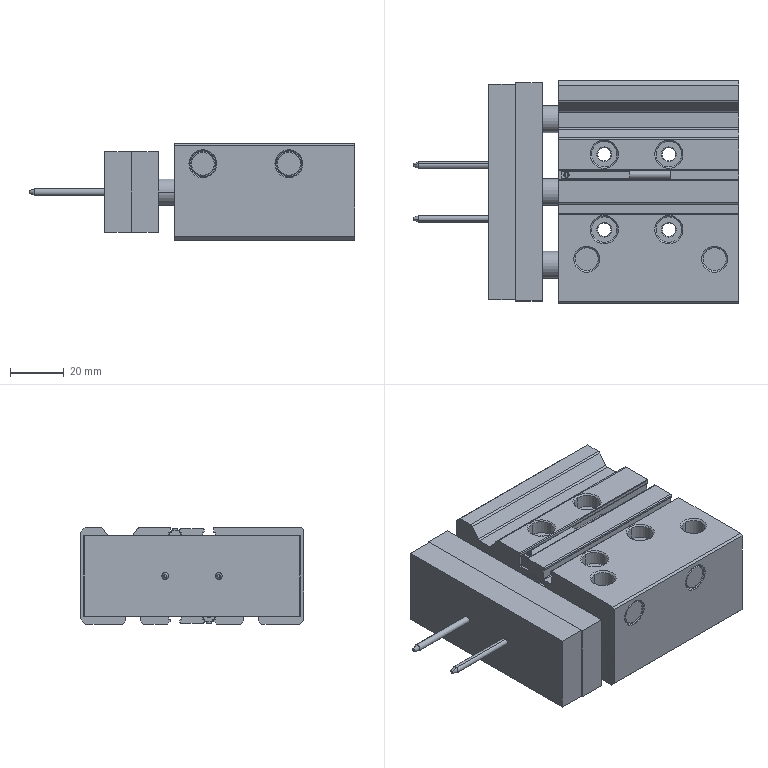Part | SolidWorks | 7 solids | 467 faces | box 121 x 83 x 36 mm | volume 201271 mm3 | cylinder 193 | plane 162 | cone 110 | torus 2 | commonest cylinder face diameters 3 x25 0.8 x20 0.4 x16 4.134 x16 0.6 x14 10 x12